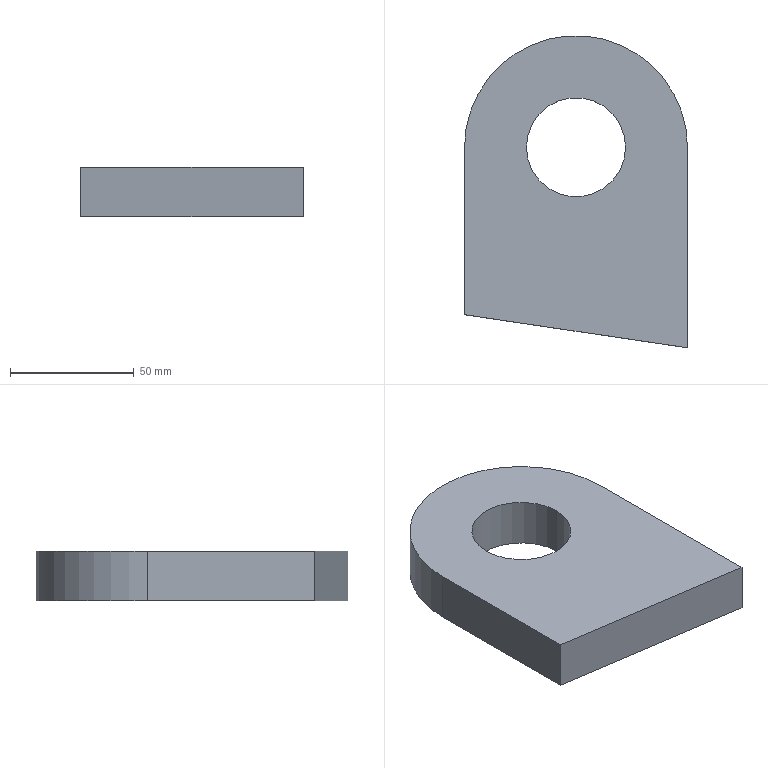Part | SolidWorks | features Extrusion 1, ICE 1 | 1 solid | 8 faces | box 90 x 126 x 20 mm | volume 172239 mm3 | plane 5 | cylinder 3 | commonest cylinder face diameters 40 x2 90 x1
STEP:
#1=CARTESIAN_POINT('',(-25.,81.,20.));
#2=VERTEX_POINT('',#1);
#3=CARTESIAN_POINT('',(-65.,81.,20.));
#4=VERTEX_POINT('',#3);
#5=CARTESIAN_POINT('',(-45.,81.,20.));
#6=DIRECTION('',(0.,0.,-1.));
#7=DIRECTION('',(-1.,0.,0.));
#8=AXIS2_PLACEMENT_3D('',#5,#6,#7);
#9=CIRCLE('',#8,20.);
#10=EDGE_CURVE('',#2,#4,#9,.T.);
#11=ORIENTED_EDGE('',*,*,#10,.F.);
#12=CARTESIAN_POINT('',(-25.,81.,0.));
#13=VERTEX_POINT('',#12);
#14=CARTESIAN_POINT('',(-25.,81.,20.));
#15=DIRECTION('',(0.,0.,-1.));
#16=VECTOR('',#15,1000.);
#17=LINE('',#14,#16);
#18=EDGE_CURVE('',#2,#13,#17,.T.);
#19=ORIENTED_EDGE('',*,*,#18,.T.);
#20=CARTESIAN_POINT('',(-65.,81.,0.));
#21=VERTEX_POINT('',#20);
#22=CARTESIAN_POINT('',(-45.,81.,0.));
#23=DIRECTION('',(0.,0.,-1.));
#24=DIRECTION('',(-1.,0.,0.));
#25=AXIS2_PLACEMENT_3D('',#22,#23,#24);
#26=CIRCLE('',#25,20.);
#27=EDGE_CURVE('',#13,#21,#26,.T.);
#28=ORIENTED_EDGE('',*,*,#27,.T.);
#29=CARTESIAN_POINT('',(-65.,81.,20.));
#30=DIRECTION('',(0.,0.,-1.));
#31=VECTOR('',#30,1000.);
#32=LINE('',#29,#31);
#33=EDGE_CURVE('',#4,#21,#32,.T.);
#34=ORIENTED_EDGE('',*,*,#33,.F.);
#35=EDGE_LOOP('',(#11,#19,#28,#34));
#36=FACE_OUTER_BOUND('',#35,.T.);
#37=CARTESIAN_POINT('',(-45.,81.,20.));
#38=DIRECTION('',(0.,0.,-1.));
#39=DIRECTION('',(-1.,0.,0.));
#40=AXIS2_PLACEMENT_3D('',#37,#38,#39);
#41=CYLINDRICAL_SURFACE('',#40,20.);
#42=ADVANCED_FACE('',(#36),#41,.F.);
#43=CARTESIAN_POINT('',(-90.,13.384,0.));
#44=VERTEX_POINT('',#43);
#45=CARTESIAN_POINT('',(0.,0.,0.));
#46=VERTEX_POINT('',#45);
#47=CARTESIAN_POINT('',(-90.,13.384,0.));
#48=DIRECTION('',(0.9891,-0.1471,0.));
#49=VECTOR('',#48,1000.);
#50=LINE('',#47,#49);
#51=EDGE_CURVE('',#44,#46,#50,.T.);
#52=ORIENTED_EDGE('',*,*,#51,.T.);
#53=CARTESIAN_POINT('',(0.,0.,20.));
#54=VERTEX_POINT('',#53);
#55=CARTESIAN_POINT('',(0.,0.,20.));
#56=DIRECTION('',(0.,0.,-1.));
#57=VECTOR('',#56,1000.);
#58=LINE('',#55,#57);
#59=EDGE_CURVE('',#54,#46,#58,.T.);
#60=ORIENTED_EDGE('',*,*,#59,.F.);
#61=CARTESIAN_POINT('',(-90.,13.384,20.));
#62=VERTEX_POINT('',#61);
#63=CARTESIAN_POINT('',(-90.,13.384,20.));
#64=DIRECTION('',(0.9891,-0.1471,0.));
#65=VECTOR('',#64,1000.);
#66=LINE('',#63,#65);
#67=EDGE_CURVE('',#62,#54,#66,.T.);
#68=ORIENTED_EDGE('',*,*,#67,.F.);
#69=CARTESIAN_POINT('',(-90.,13.384,20.));
#70=DIRECTION('',(0.,0.,-1.));
#71=VECTOR('',#70,1000.);
#72=LINE('',#69,#71);
#73=EDGE_CURVE('',#62,#44,#72,.T.);
#74=ORIENTED_EDGE('',*,*,#73,.T.);
#75=EDGE_LOOP('',(#52,#60,#68,#74));
#76=FACE_OUTER_BOUND('',#75,.T.);
#77=CARTESIAN_POINT('',(-90.,13.384,20.));
#78=DIRECTION('',(0.1471,0.9891,0.));
#79=DIRECTION('',(-0.9891,0.1471,0.));
#80=AXIS2_PLACEMENT_3D('',#77,#78,#79);
#81=PLANE('',#80);
#82=ADVANCED_FACE('',(#76),#81,.F.);
#83=CARTESIAN_POINT('',(0.,81.,0.));
#84=VERTEX_POINT('',#83);
#85=CARTESIAN_POINT('',(0.,0.,0.));
#86=DIRECTION('',(0.,1.,0.));
#87=VECTOR('',#86,1000.);
#88=LINE('',#85,#87);
#89=EDGE_CURVE('',#46,#84,#88,.T.);
#90=ORIENTED_EDGE('',*,*,#89,.T.);
#91=CARTESIAN_POINT('',(0.,81.,20.));
#92=VERTEX_POINT('',#91);
#93=CARTESIAN_POINT('',(0.,81.,20.));
#94=DIRECTION('',(0.,0.,-1.));
#95=VECTOR('',#94,1000.);
#96=LINE('',#93,#95);
#97=EDGE_CURVE('',#92,#84,#96,.T.);
#98=ORIENTED_EDGE('',*,*,#97,.F.);
#99=CARTESIAN_POINT('',(0.,0.,20.));
#100=DIRECTION('',(0.,1.,0.));
#101=VECTOR('',#100,1000.);
#102=LINE('',#99,#101);
#103=EDGE_CURVE('',#54,#92,#102,.T.);
#104=ORIENTED_EDGE('',*,*,#103,.F.);
#105=ORIENTED_EDGE('',*,*,#59,.T.);
#106=EDGE_LOOP('',(#90,#98,#104,#105));
#107=FACE_OUTER_BOUND('',#106,.T.);
#108=CARTESIAN_POINT('',(0.,0.,20.));
#109=DIRECTION('',(-1.,0.,0.));
#110=DIRECTION('',(0.,-1.,0.));
#111=AXIS2_PLACEMENT_3D('',#108,#109,#110);
#112=PLANE('',#111);
#113=ADVANCED_FACE('',(#107),#112,.F.);
#114=CARTESIAN_POINT('',(-90.,81.,0.));
#115=VERTEX_POINT('',#114);
#116=CARTESIAN_POINT('',(-45.,81.,0.));
#117=DIRECTION('',(0.,0.,1.));
#118=DIRECTION('',(1.,0.,0.));
#119=AXIS2_PLACEMENT_3D('',#116,#117,#118);
#120=CIRCLE('',#119,45.);
#121=EDGE_CURVE('',#84,#115,#120,.T.);
#122=ORIENTED_EDGE('',*,*,#121,.T.);
#123=CARTESIAN_POINT('',(-90.,81.,20.));
#124=VERTEX_POINT('',#123);
#125=CARTESIAN_POINT('',(-90.,81.,20.));
#126=DIRECTION('',(0.,0.,-1.));
#127=VECTOR('',#126,1000.);
#128=LINE('',#125,#127);
#129=EDGE_CURVE('',#124,#115,#128,.T.);
#130=ORIENTED_EDGE('',*,*,#129,.F.);
#131=CARTESIAN_POINT('',(-45.,81.,20.));
#132=DIRECTION('',(0.,0.,1.));
#133=DIRECTION('',(1.,0.,0.));
#134=AXIS2_PLACEMENT_3D('',#131,#132,#133);
#135=CIRCLE('',#134,45.);
#136=EDGE_CURVE('',#92,#124,#135,.T.);
#137=ORIENTED_EDGE('',*,*,#136,.F.);
#138=ORIENTED_EDGE('',*,*,#97,.T.);
#139=EDGE_LOOP('',(#122,#130,#137,#138));
#140=FACE_OUTER_BOUND('',#139,.T.);
#141=CARTESIAN_POINT('',(-45.,81.,20.));
#142=DIRECTION('',(0.,0.,-1.));
#143=DIRECTION('',(-1.,0.,0.));
#144=AXIS2_PLACEMENT_3D('',#141,#142,#143);
#145=CYLINDRICAL_SURFACE('',#144,45.);
#146=ADVANCED_FACE('',(#140),#145,.T.);
#147=CARTESIAN_POINT('',(-90.,81.,0.));
#148=DIRECTION('',(0.,-1.,0.));
#149=VECTOR('',#148,1000.);
#150=LINE('',#147,#149);
#151=EDGE_CURVE('',#115,#44,#150,.T.);
#152=ORIENTED_EDGE('',*,*,#151,.T.);
#153=ORIENTED_EDGE('',*,*,#73,.F.);
#154=CARTESIAN_POINT('',(-90.,81.,20.));
#155=DIRECTION('',(0.,-1.,0.));
#156=VECTOR('',#155,1000.);
#157=LINE('',#154,#156);
#158=EDGE_CURVE('',#124,#62,#157,.T.);
#159=ORIENTED_EDGE('',*,*,#158,.F.);
#160=ORIENTED_EDGE('',*,*,#129,.T.);
#161=EDGE_LOOP('',(#152,#153,#159,#160));
#162=FACE_OUTER_BOUND('',#161,.T.);
#163=CARTESIAN_POINT('',(-90.,81.,20.));
#164=DIRECTION('',(1.,0.,0.));
#165=DIRECTION('',(0.,1.,0.));
#166=AXIS2_PLACEMENT_3D('',#163,#164,#165);
#167=PLANE('',#166);
#168=ADVANCED_FACE('',(#162),#167,.F.);
#169=CARTESIAN_POINT('',(-45.,81.,20.));
#170=DIRECTION('',(0.,0.,-1.));
#171=DIRECTION('',(-1.,0.,0.));
#172=AXIS2_PLACEMENT_3D('',#169,#170,#171);
#173=CIRCLE('',#172,20.);
#174=EDGE_CURVE('',#4,#2,#173,.T.);
#175=ORIENTED_EDGE('',*,*,#174,.T.);
#176=ORIENTED_EDGE('',*,*,#10,.T.);
#177=EDGE_LOOP('',(#175,#176));
#178=FACE_BOUND('',#177,.T.);
#179=ORIENTED_EDGE('',*,*,#67,.T.);
#180=ORIENTED_EDGE('',*,*,#103,.T.);
#181=ORIENTED_EDGE('',*,*,#136,.T.);
#182=ORIENTED_EDGE('',*,*,#158,.T.);
#183=EDGE_LOOP('',(#179,#180,#181,#182));
#184=FACE_OUTER_BOUND('',#183,.T.);
#185=CARTESIAN_POINT('',(-45.,81.,20.));
#186=DIRECTION('',(0.,0.,1.));
#187=DIRECTION('',(1.,0.,0.));
#188=AXIS2_PLACEMENT_3D('',#185,#186,#187);
#189=PLANE('',#188);
#190=ADVANCED_FACE('',(#178,#184),#189,.T.);
#191=CARTESIAN_POINT('',(-45.,81.,0.));
#192=DIRECTION('',(0.,0.,-1.));
#193=DIRECTION('',(-1.,0.,0.));
#194=AXIS2_PLACEMENT_3D('',#191,#192,#193);
#195=CIRCLE('',#194,20.);
#196=EDGE_CURVE('',#21,#13,#195,.T.);
#197=ORIENTED_EDGE('',*,*,#196,.F.);
#198=ORIENTED_EDGE('',*,*,#27,.F.);
#199=EDGE_LOOP('',(#197,#198));
#200=FACE_BOUND('',#199,.T.);
#201=ORIENTED_EDGE('',*,*,#51,.F.);
#202=ORIENTED_EDGE('',*,*,#151,.F.);
#203=ORIENTED_EDGE('',*,*,#121,.F.);
#204=ORIENTED_EDGE('',*,*,#89,.F.);
#205=EDGE_LOOP('',(#201,#202,#203,#204));
#206=FACE_OUTER_BOUND('',#205,.T.);
#207=CARTESIAN_POINT('',(-45.,81.,0.));
#208=DIRECTION('',(0.,0.,1.));
#209=DIRECTION('',(1.,0.,0.));
#210=AXIS2_PLACEMENT_3D('',#207,#208,#209);
#211=PLANE('',#210);
#212=ADVANCED_FACE('',(#200,#206),#211,.F.);
#213=ORIENTED_EDGE('',*,*,#18,.F.);
#214=ORIENTED_EDGE('',*,*,#174,.F.);
#215=ORIENTED_EDGE('',*,*,#33,.T.);
#216=ORIENTED_EDGE('',*,*,#196,.T.);
#217=EDGE_LOOP('',(#213,#214,#215,#216));
#218=FACE_OUTER_BOUND('',#217,.T.);
#219=CARTESIAN_POINT('',(-45.,81.,20.));
#220=DIRECTION('',(0.,0.,-1.));
#221=DIRECTION('',(-1.,0.,0.));
#222=AXIS2_PLACEMENT_3D('',#219,#220,#221);
#223=CYLINDRICAL_SURFACE('',#222,20.);
#224=ADVANCED_FACE('',(#218),#223,.F.);
#225=CLOSED_SHELL('',(#42,#82,#113,#146,#168,#190,#212,#224));
#226=MANIFOLD_SOLID_BREP('',#225);
#227=CARTESIAN_POINT('',(0.,0.,0.));
#228=DIRECTION('',(0.,0.,1.));
#229=DIRECTION('',(1.,0.,0.));
#230=AXIS2_PLACEMENT_3D('',#227,#228,#229);
#231=(LENGTH_UNIT()NAMED_UNIT(*)SI_UNIT(.MILLI.,.METRE.));
#232=UNCERTAINTY_MEASURE_WITH_UNIT(LENGTH_MEASURE(0.00001),#231,'','');
#233=(NAMED_UNIT(*)PLANE_ANGLE_UNIT()SI_UNIT($,.RADIAN.));
#234=(NAMED_UNIT(*)SI_UNIT($,.STERADIAN.)SOLID_ANGLE_UNIT());
#235=(GEOMETRIC_REPRESENTATION_CONTEXT(3)GLOBAL_UNCERTAINTY_ASSIGNED_CONTEXT((#232))GLOBAL_UNIT_ASSIGNED_CONTEXT((#231,#233,#234))REPRESENTATION_CONTEXT('',''));
#236=ADVANCED_BREP_SHAPE_REPRESENTATION('',(#226,#230),#235);